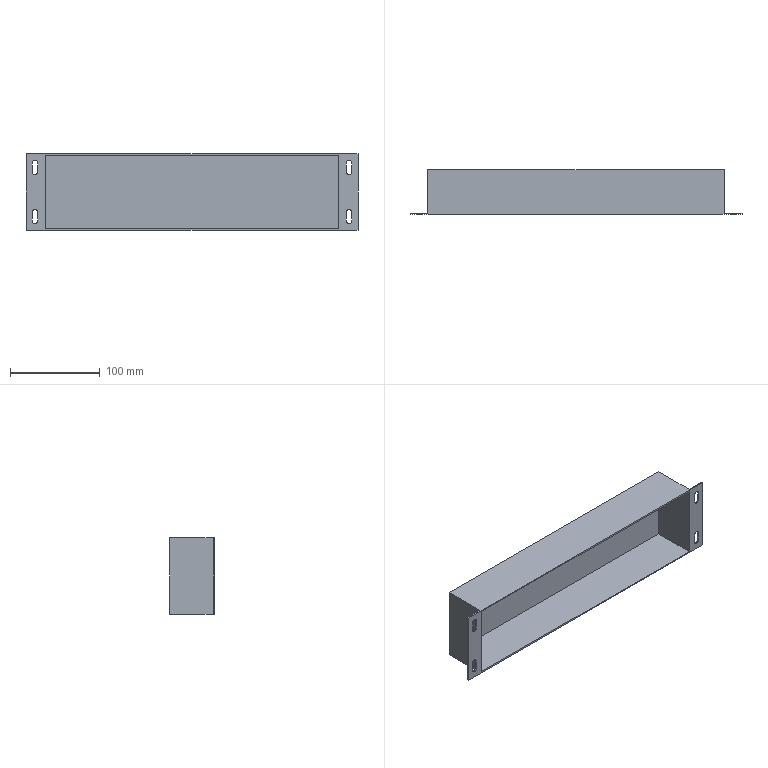Part | STEP file | 601-01-0066 | 1 solid | 35 faces | box 370 x 50 x 85 mm | volume 106591 mm3 | plane 23 | cylinder 12 | commonest cylinder face diameters 6 x12